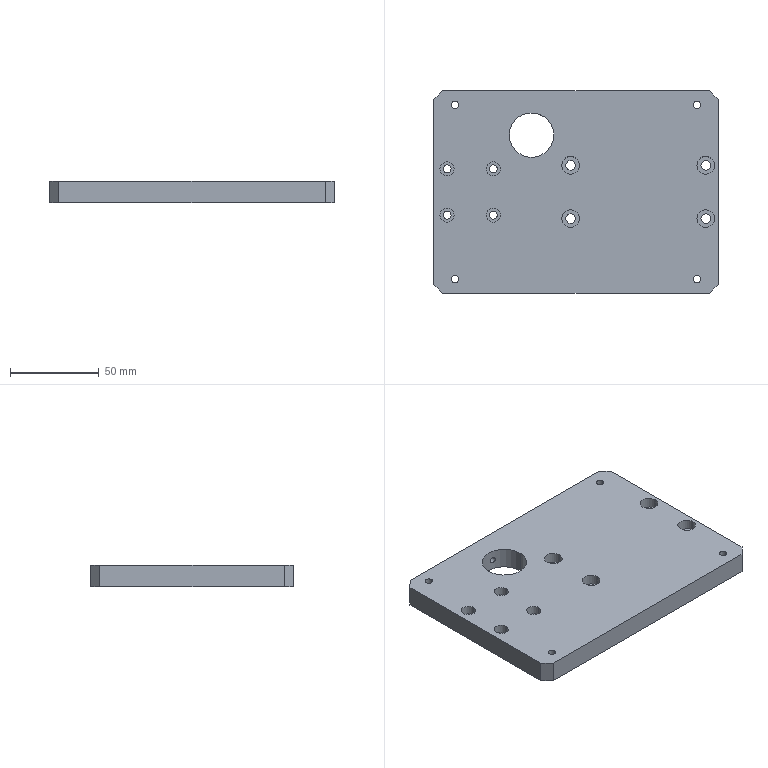Part | STEP file | ASND-0110-Body 1-9 | 1 solid | 66 faces | box 160 x 114 x 12 mm | volume 207606 mm3 | cylinder 46 | plane 18 | cone 2 | commonest cylinder face diameters 4.134 x8 4.5 x8 5.5 x8 8 x8 10 x8 3.242 x4